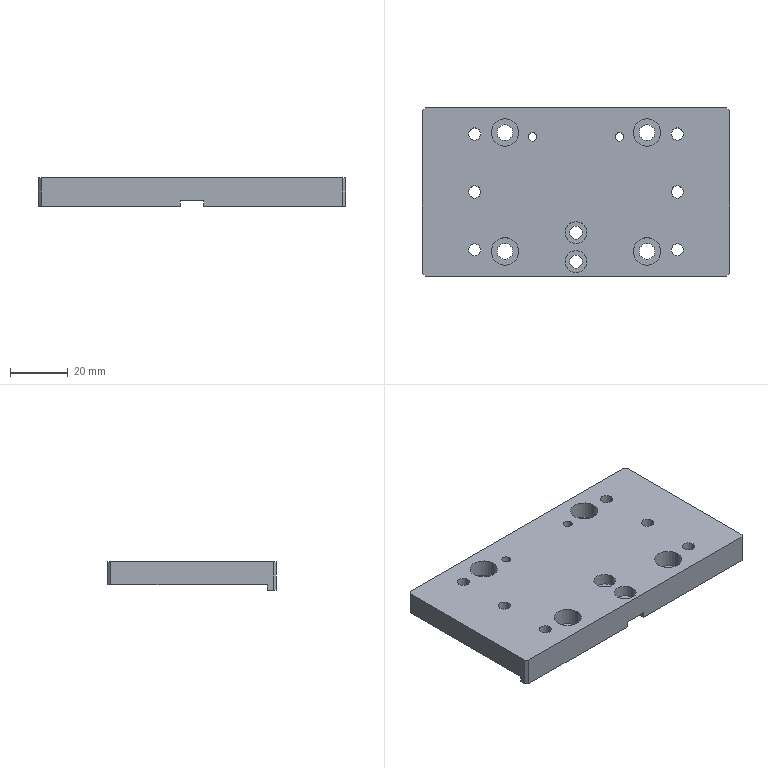Part | STEP file | PN_0062 Mount electronic clip s horizontal manipulator flange plate | 1 solid | 62 faces | box 106 x 58 x 10 mm | volume 46604 mm3 | cylinder 40 | plane 22 | commonest cylinder face diameters 4.2 x12 5.5 x8 9.5 x8 3 x4 4.5 x4 7.5 x4